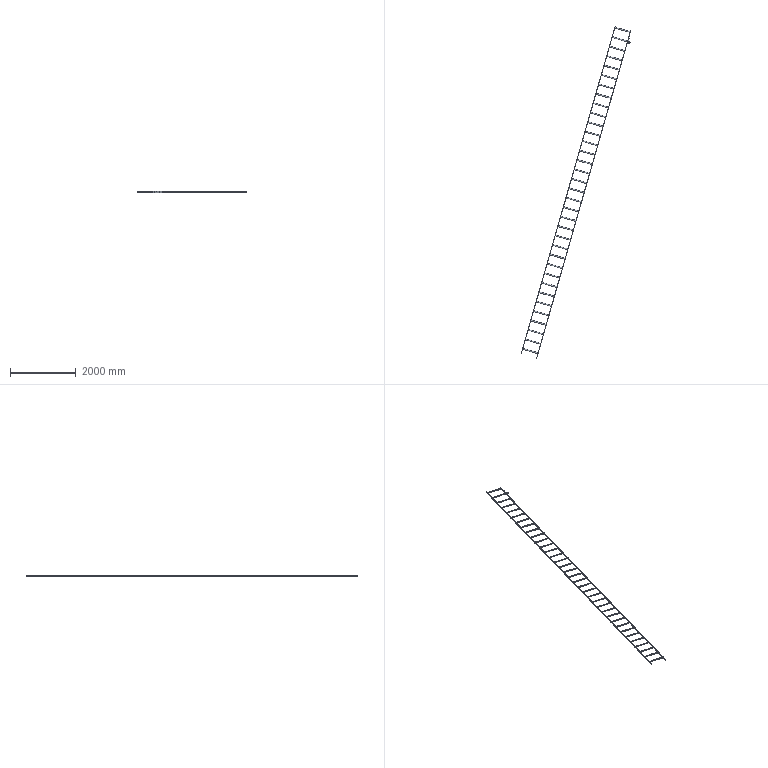Part | SolidWorks | features WeldMemberFeat 2, Chamfer 1, LPattern 1, Sweep 1, WeldCornerFeat 1, WeldmentFeature 1 | 38 solids | 237 faces | box 3347 x 10135 x 40 mm | volume 8856041 mm3 | cylinder 146 | plane 84 | torus 5 | cone 2 | commonest cylinder face diameters 20.8 x70 26.8 x70 12 x6